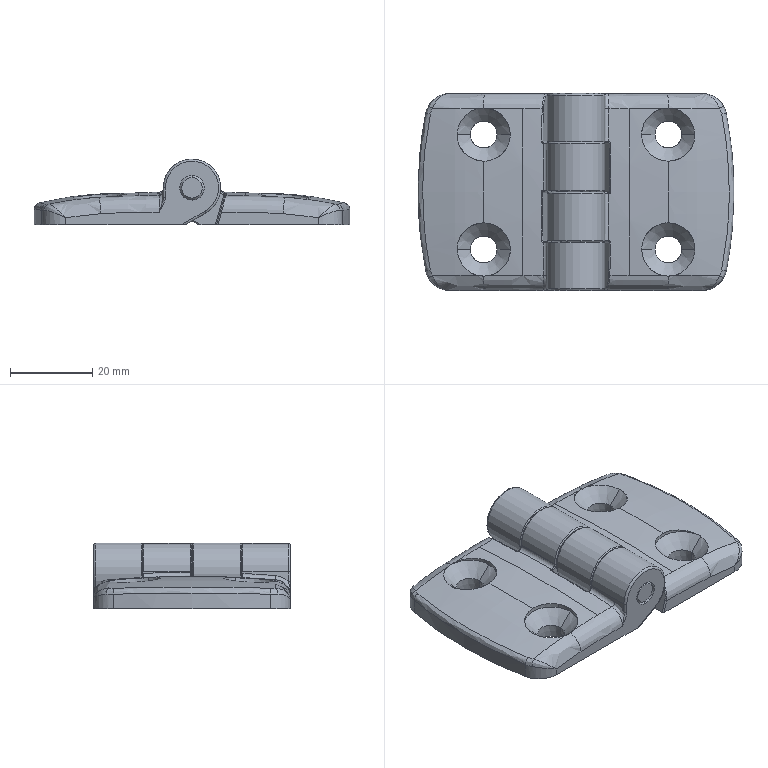Part | SolidWorks | 3 solids | 168 faces | box 77 x 48 x 16 mm | volume 26381 mm3 | cylinder 52 | spline 40 | plane 26 | torus 26 | cone 20 | sphere 4 | commonest cylinder face diameters 0.6 x20 6 x10 13 x8 1 x4 12 x4 14 x4